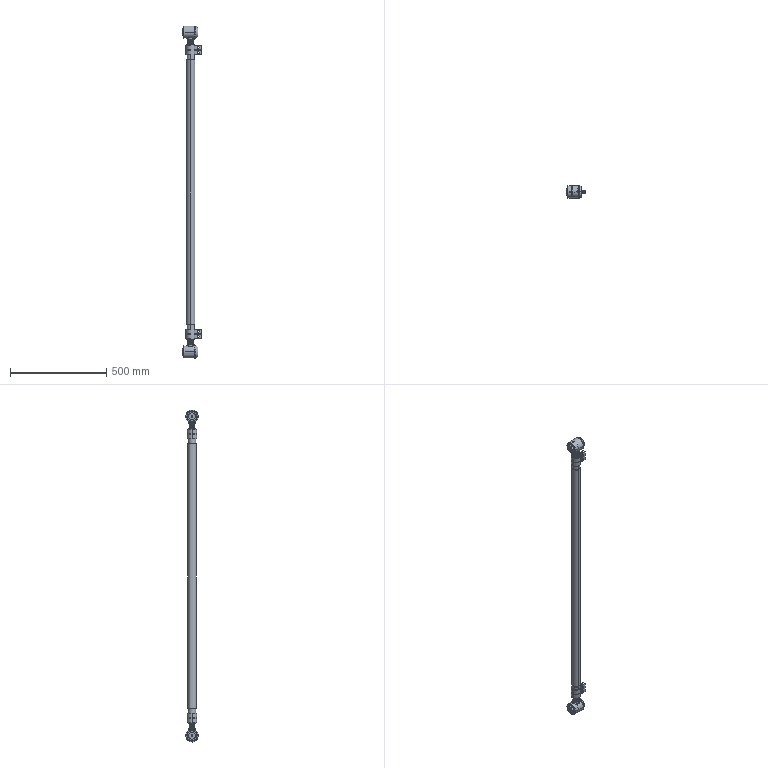Part | SolidWorks | features ReferencePattern 2, MirrorCompFeat 1 | 13 solids | 484 faces | box 103 x 64 x 1722 mm | volume 2094489 mm3 | cylinder 333 | plane 86 | cone 51 | spline 8 | sphere 6 | commonest cylinder face diameters 30 x212 11 x16 40 x16 50 x10 4 x8 12 x8